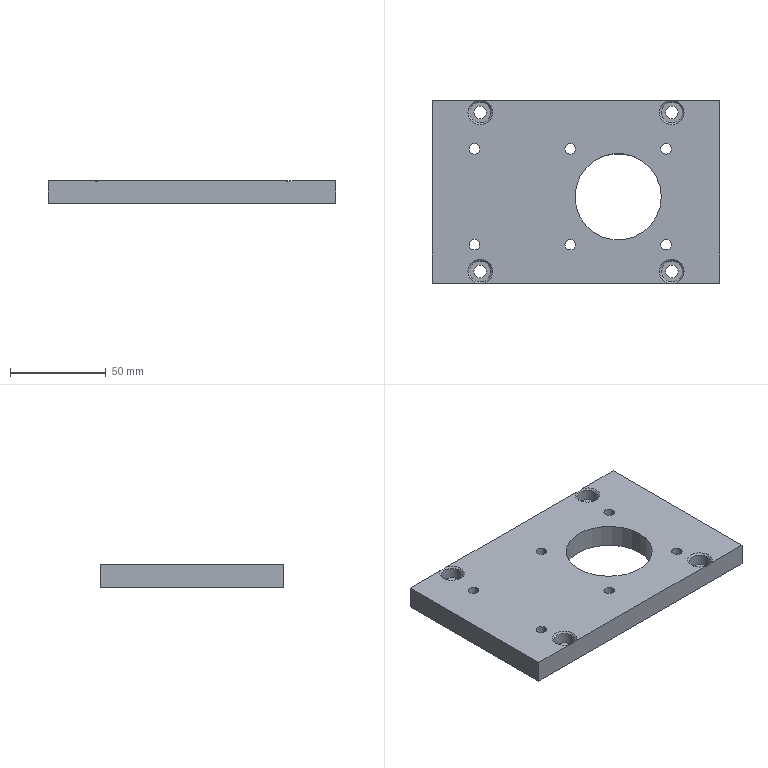Part | SolidWorks | features HoleWzd 2, Cut 1, Extrusion 1 | 1 solid | 78 faces | box 150 x 95 x 12 mm | volume 144976 mm3 | cylinder 42 | cone 20 | plane 16 | commonest cylinder face diameters 5.5 x12 10 x12 6.6 x8 11 x8 45 x2